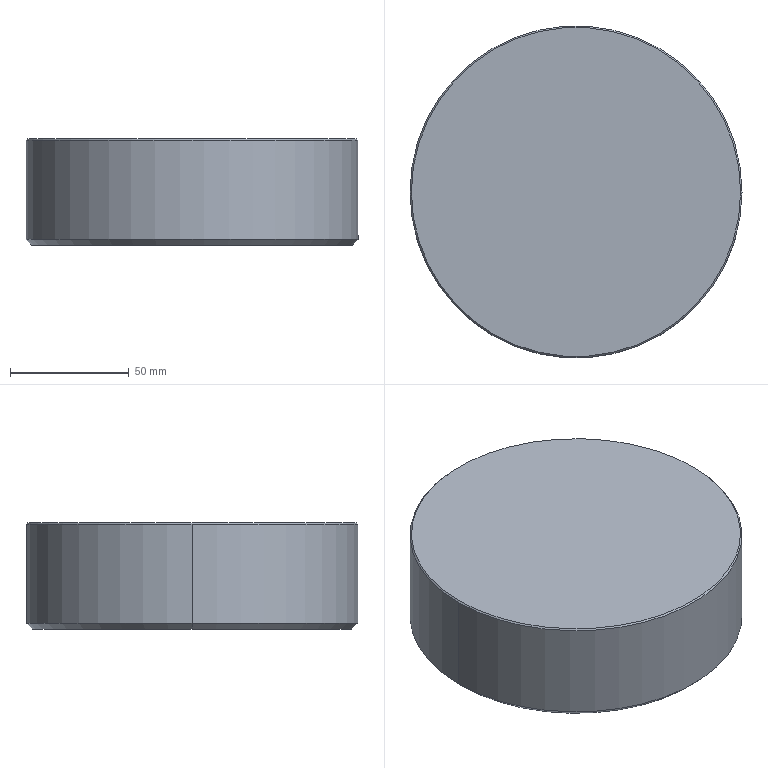Part | SolidWorks | features BaseBody 1 | 1 solid | 13 faces | box 140 x 140 x 45 mm | volume 200339 mm3 | cone 6 | cylinder 4 | plane 3 | commonest cylinder face diameters 125 x2 140 x2
STEP:
#1=CARTESIAN_POINT('',(69.4,0.,45.));
#2=VERTEX_POINT('',#1);
#3=CARTESIAN_POINT('',(-69.4,0.,45.));
#4=VERTEX_POINT('',#3);
#5=CARTESIAN_POINT('',(0.,0.,45.));
#6=DIRECTION('',(0.,0.,1.));
#7=DIRECTION('',(-1.,0.,0.));
#8=AXIS2_PLACEMENT_3D('',#5,#6,#7);
#9=CIRCLE('',#8,69.4);
#10=EDGE_CURVE('',#2,#4,#9,.T.);
#11=ORIENTED_EDGE('',*,*,#10,.F.);
#12=CARTESIAN_POINT('',(70.,0.,44.4));
#13=VERTEX_POINT('',#12);
#14=CARTESIAN_POINT('',(70.,0.,44.4));
#15=DIRECTION('',(0.7071,0.,-0.7071));
#16=VECTOR('',#15,1000.);
#17=LINE('',#14,#16);
#18=EDGE_CURVE('',#2,#13,#17,.T.);
#19=ORIENTED_EDGE('',*,*,#18,.T.);
#20=CARTESIAN_POINT('',(-70.,0.,44.4));
#21=VERTEX_POINT('',#20);
#22=CARTESIAN_POINT('',(0.,0.,44.4));
#23=DIRECTION('',(0.,0.,1.));
#24=DIRECTION('',(-1.,0.,0.));
#25=AXIS2_PLACEMENT_3D('',#22,#23,#24);
#26=CIRCLE('',#25,70.);
#27=EDGE_CURVE('',#13,#21,#26,.T.);
#28=ORIENTED_EDGE('',*,*,#27,.T.);
#29=CARTESIAN_POINT('',(-70.,0.,44.4));
#30=DIRECTION('',(-0.7071,0.,-0.7071));
#31=VECTOR('',#30,1000.);
#32=LINE('',#29,#31);
#33=EDGE_CURVE('',#4,#21,#32,.T.);
#34=ORIENTED_EDGE('',*,*,#33,.F.);
#35=EDGE_LOOP('',(#11,#19,#28,#34));
#36=FACE_OUTER_BOUND('',#35,.T.);
#37=CARTESIAN_POINT('',(0.,0.,44.4));
#38=DIRECTION('',(0.,0.,-1.));
#39=DIRECTION('',(-1.,0.,0.));
#40=AXIS2_PLACEMENT_3D('',#37,#38,#39);
#41=CONICAL_SURFACE('',#40,70.,0.7854);
#42=ADVANCED_FACE('',(#36),#41,.T.);
#43=ORIENTED_EDGE('',*,*,#27,.F.);
#44=CARTESIAN_POINT('',(70.,0.,2.5));
#45=VERTEX_POINT('',#44);
#46=CARTESIAN_POINT('',(70.,0.,40.));
#47=DIRECTION('',(0.,0.,-1.));
#48=VECTOR('',#47,1000.);
#49=LINE('',#46,#48);
#50=EDGE_CURVE('',#13,#45,#49,.T.);
#51=ORIENTED_EDGE('',*,*,#50,.T.);
#52=CARTESIAN_POINT('',(-70.,0.,2.5));
#53=VERTEX_POINT('',#52);
#54=CARTESIAN_POINT('',(0.,0.,2.5));
#55=DIRECTION('',(0.,0.,1.));
#56=DIRECTION('',(-1.,0.,0.));
#57=AXIS2_PLACEMENT_3D('',#54,#55,#56);
#58=CIRCLE('',#57,70.);
#59=EDGE_CURVE('',#45,#53,#58,.T.);
#60=ORIENTED_EDGE('',*,*,#59,.T.);
#61=CARTESIAN_POINT('',(-70.,0.,40.));
#62=DIRECTION('',(0.,0.,-1.));
#63=VECTOR('',#62,1000.);
#64=LINE('',#61,#63);
#65=EDGE_CURVE('',#21,#53,#64,.T.);
#66=ORIENTED_EDGE('',*,*,#65,.F.);
#67=EDGE_LOOP('',(#43,#51,#60,#66));
#68=FACE_OUTER_BOUND('',#67,.T.);
#69=CARTESIAN_POINT('',(0.,0.,40.));
#70=DIRECTION('',(0.,0.,-1.));
#71=DIRECTION('',(-1.,0.,0.));
#72=AXIS2_PLACEMENT_3D('',#69,#70,#71);
#73=CYLINDRICAL_SURFACE('',#72,70.);
#74=ADVANCED_FACE('',(#68),#73,.T.);
#75=CARTESIAN_POINT('',(67.5,0.,0.));
#76=VERTEX_POINT('',#75);
#77=CARTESIAN_POINT('',(-67.5,0.,0.));
#78=VERTEX_POINT('',#77);
#79=CARTESIAN_POINT('',(0.,0.,0.));
#80=DIRECTION('',(0.,0.,1.));
#81=DIRECTION('',(1.,0.,0.));
#82=AXIS2_PLACEMENT_3D('',#79,#80,#81);
#83=CIRCLE('',#82,67.5);
#84=EDGE_CURVE('',#76,#78,#83,.T.);
#85=ORIENTED_EDGE('',*,*,#84,.T.);
#86=CARTESIAN_POINT('',(-70.,0.,2.5));
#87=DIRECTION('',(-0.7071,0.,0.7071));
#88=VECTOR('',#87,1000.);
#89=LINE('',#86,#88);
#90=EDGE_CURVE('',#78,#53,#89,.T.);
#91=ORIENTED_EDGE('',*,*,#90,.T.);
#92=ORIENTED_EDGE('',*,*,#59,.F.);
#93=CARTESIAN_POINT('',(70.,0.,2.5));
#94=DIRECTION('',(0.7071,0.,0.7071));
#95=VECTOR('',#94,1000.);
#96=LINE('',#93,#95);
#97=EDGE_CURVE('',#76,#45,#96,.T.);
#98=ORIENTED_EDGE('',*,*,#97,.F.);
#99=EDGE_LOOP('',(#85,#91,#92,#98));
#100=FACE_OUTER_BOUND('',#99,.T.);
#101=CARTESIAN_POINT('',(0.,0.,2.5));
#102=DIRECTION('',(0.,0.,1.));
#103=DIRECTION('',(1.,0.,0.));
#104=AXIS2_PLACEMENT_3D('',#101,#102,#103);
#105=CONICAL_SURFACE('',#104,70.,0.7854);
#106=ADVANCED_FACE('',(#100),#105,.T.);
#107=CARTESIAN_POINT('',(62.5,0.,0.6));
#108=VERTEX_POINT('',#107);
#109=CARTESIAN_POINT('',(-62.5,0.,0.6));
#110=VERTEX_POINT('',#109);
#111=CARTESIAN_POINT('',(0.,0.,0.6));
#112=DIRECTION('',(0.,0.,-1.));
#113=DIRECTION('',(1.,0.,0.));
#114=AXIS2_PLACEMENT_3D('',#111,#112,#113);
#115=CIRCLE('',#114,62.5);
#116=EDGE_CURVE('',#108,#110,#115,.T.);
#117=ORIENTED_EDGE('',*,*,#116,.F.);
#118=CARTESIAN_POINT('',(63.1,0.,0.));
#119=VERTEX_POINT('',#118);
#120=CARTESIAN_POINT('',(63.1,0.,0.));
#121=DIRECTION('',(0.7071,0.,-0.7071));
#122=VECTOR('',#121,1000.);
#123=LINE('',#120,#122);
#124=EDGE_CURVE('',#108,#119,#123,.T.);
#125=ORIENTED_EDGE('',*,*,#124,.T.);
#126=CARTESIAN_POINT('',(-63.1,0.,0.));
#127=VERTEX_POINT('',#126);
#128=CARTESIAN_POINT('',(0.,0.,0.));
#129=DIRECTION('',(0.,0.,-1.));
#130=DIRECTION('',(-1.,0.,0.));
#131=AXIS2_PLACEMENT_3D('',#128,#129,#130);
#132=CIRCLE('',#131,63.1);
#133=EDGE_CURVE('',#119,#127,#132,.T.);
#134=ORIENTED_EDGE('',*,*,#133,.T.);
#135=CARTESIAN_POINT('',(-63.1,0.,0.));
#136=DIRECTION('',(-0.7071,0.,-0.7071));
#137=VECTOR('',#136,1000.);
#138=LINE('',#135,#137);
#139=EDGE_CURVE('',#110,#127,#138,.T.);
#140=ORIENTED_EDGE('',*,*,#139,.F.);
#141=EDGE_LOOP('',(#117,#125,#134,#140));
#142=FACE_OUTER_BOUND('',#141,.T.);
#143=CARTESIAN_POINT('',(0.,0.,0.));
#144=DIRECTION('',(0.,0.,-1.));
#145=DIRECTION('',(-1.,0.,0.));
#146=AXIS2_PLACEMENT_3D('',#143,#144,#145);
#147=CONICAL_SURFACE('',#146,63.1,0.7854);
#148=ADVANCED_FACE('',(#142),#147,.F.);
#149=CARTESIAN_POINT('',(62.5,0.,40.));
#150=VERTEX_POINT('',#149);
#151=CARTESIAN_POINT('',(-62.5,0.,40.));
#152=VERTEX_POINT('',#151);
#153=CARTESIAN_POINT('',(0.,0.,40.));
#154=DIRECTION('',(0.,0.,-1.));
#155=DIRECTION('',(-1.,0.,0.));
#156=AXIS2_PLACEMENT_3D('',#153,#154,#155);
#157=CIRCLE('',#156,62.5);
#158=EDGE_CURVE('',#150,#152,#157,.T.);
#159=ORIENTED_EDGE('',*,*,#158,.F.);
#160=CARTESIAN_POINT('',(62.5,0.,40.));
#161=DIRECTION('',(0.,0.,-1.));
#162=VECTOR('',#161,1000.);
#163=LINE('',#160,#162);
#164=EDGE_CURVE('',#150,#108,#163,.T.);
#165=ORIENTED_EDGE('',*,*,#164,.T.);
#166=ORIENTED_EDGE('',*,*,#116,.T.);
#167=CARTESIAN_POINT('',(-62.5,0.,40.));
#168=DIRECTION('',(0.,0.,-1.));
#169=VECTOR('',#168,1000.);
#170=LINE('',#167,#169);
#171=EDGE_CURVE('',#152,#110,#170,.T.);
#172=ORIENTED_EDGE('',*,*,#171,.F.);
#173=EDGE_LOOP('',(#159,#165,#166,#172));
#174=FACE_OUTER_BOUND('',#173,.T.);
#175=CARTESIAN_POINT('',(0.,0.,40.));
#176=DIRECTION('',(0.,0.,-1.));
#177=DIRECTION('',(-1.,0.,0.));
#178=AXIS2_PLACEMENT_3D('',#175,#176,#177);
#179=CYLINDRICAL_SURFACE('',#178,62.5);
#180=ADVANCED_FACE('',(#174),#179,.F.);
#181=CARTESIAN_POINT('',(0.,0.,45.));
#182=DIRECTION('',(0.,0.,1.));
#183=DIRECTION('',(-1.,0.,0.));
#184=AXIS2_PLACEMENT_3D('',#181,#182,#183);
#185=CIRCLE('',#184,69.4);
#186=EDGE_CURVE('',#4,#2,#185,.T.);
#187=ORIENTED_EDGE('',*,*,#186,.T.);
#188=ORIENTED_EDGE('',*,*,#10,.T.);
#189=EDGE_LOOP('',(#187,#188));
#190=FACE_OUTER_BOUND('',#189,.T.);
#191=CARTESIAN_POINT('',(0.,0.,45.));
#192=DIRECTION('',(0.,0.,1.));
#193=DIRECTION('',(1.,0.,0.));
#194=AXIS2_PLACEMENT_3D('',#191,#192,#193);
#195=PLANE('',#194);
#196=ADVANCED_FACE('',(#190),#195,.T.);
#197=ORIENTED_EDGE('',*,*,#18,.F.);
#198=ORIENTED_EDGE('',*,*,#186,.F.);
#199=ORIENTED_EDGE('',*,*,#33,.T.);
#200=CARTESIAN_POINT('',(0.,0.,44.4));
#201=DIRECTION('',(0.,0.,1.));
#202=DIRECTION('',(-1.,0.,0.));
#203=AXIS2_PLACEMENT_3D('',#200,#201,#202);
#204=CIRCLE('',#203,70.);
#205=EDGE_CURVE('',#21,#13,#204,.T.);
#206=ORIENTED_EDGE('',*,*,#205,.T.);
#207=EDGE_LOOP('',(#197,#198,#199,#206));
#208=FACE_OUTER_BOUND('',#207,.T.);
#209=CARTESIAN_POINT('',(0.,0.,44.4));
#210=DIRECTION('',(0.,0.,-1.));
#211=DIRECTION('',(-1.,0.,0.));
#212=AXIS2_PLACEMENT_3D('',#209,#210,#211);
#213=CONICAL_SURFACE('',#212,70.,0.7854);
#214=ADVANCED_FACE('',(#208),#213,.T.);
#215=ORIENTED_EDGE('',*,*,#50,.F.);
#216=ORIENTED_EDGE('',*,*,#205,.F.);
#217=ORIENTED_EDGE('',*,*,#65,.T.);
#218=CARTESIAN_POINT('',(0.,0.,2.5));
#219=DIRECTION('',(0.,0.,1.));
#220=DIRECTION('',(-1.,0.,0.));
#221=AXIS2_PLACEMENT_3D('',#218,#219,#220);
#222=CIRCLE('',#221,70.);
#223=EDGE_CURVE('',#53,#45,#222,.T.);
#224=ORIENTED_EDGE('',*,*,#223,.T.);
#225=EDGE_LOOP('',(#215,#216,#217,#224));
#226=FACE_OUTER_BOUND('',#225,.T.);
#227=CARTESIAN_POINT('',(0.,0.,40.));
#228=DIRECTION('',(0.,0.,-1.));
#229=DIRECTION('',(-1.,0.,0.));
#230=AXIS2_PLACEMENT_3D('',#227,#228,#229);
#231=CYLINDRICAL_SURFACE('',#230,70.);
#232=ADVANCED_FACE('',(#226),#231,.T.);
#233=ORIENTED_EDGE('',*,*,#90,.F.);
#234=CARTESIAN_POINT('',(0.,0.,0.));
#235=DIRECTION('',(0.,0.,1.));
#236=DIRECTION('',(1.,0.,0.));
#237=AXIS2_PLACEMENT_3D('',#234,#235,#236);
#238=CIRCLE('',#237,67.5);
#239=EDGE_CURVE('',#78,#76,#238,.T.);
#240=ORIENTED_EDGE('',*,*,#239,.T.);
#241=ORIENTED_EDGE('',*,*,#97,.T.);
#242=ORIENTED_EDGE('',*,*,#223,.F.);
#243=EDGE_LOOP('',(#233,#240,#241,#242));
#244=FACE_OUTER_BOUND('',#243,.T.);
#245=CARTESIAN_POINT('',(0.,0.,2.5));
#246=DIRECTION('',(0.,0.,1.));
#247=DIRECTION('',(1.,0.,0.));
#248=AXIS2_PLACEMENT_3D('',#245,#246,#247);
#249=CONICAL_SURFACE('',#248,70.,0.7854);
#250=ADVANCED_FACE('',(#244),#249,.T.);
#251=CARTESIAN_POINT('',(0.,0.,0.));
#252=DIRECTION('',(0.,0.,-1.));
#253=DIRECTION('',(-1.,0.,0.));
#254=AXIS2_PLACEMENT_3D('',#251,#252,#253);
#255=CIRCLE('',#254,63.1);
#256=EDGE_CURVE('',#127,#119,#255,.T.);
#257=ORIENTED_EDGE('',*,*,#256,.F.);
#258=ORIENTED_EDGE('',*,*,#133,.F.);
#259=EDGE_LOOP('',(#257,#258));
#260=FACE_BOUND('',#259,.T.);
#261=ORIENTED_EDGE('',*,*,#84,.F.);
#262=ORIENTED_EDGE('',*,*,#239,.F.);
#263=EDGE_LOOP('',(#261,#262));
#264=FACE_OUTER_BOUND('',#263,.T.);
#265=CARTESIAN_POINT('',(0.,0.,0.));
#266=DIRECTION('',(0.,0.,1.));
#267=DIRECTION('',(1.,0.,0.));
#268=AXIS2_PLACEMENT_3D('',#265,#266,#267);
#269=PLANE('',#268);
#270=ADVANCED_FACE('',(#260,#264),#269,.F.);
#271=ORIENTED_EDGE('',*,*,#124,.F.);
#272=CARTESIAN_POINT('',(0.,0.,0.6));
#273=DIRECTION('',(0.,0.,-1.));
#274=DIRECTION('',(1.,0.,0.));
#275=AXIS2_PLACEMENT_3D('',#272,#273,#274);
#276=CIRCLE('',#275,62.5);
#277=EDGE_CURVE('',#110,#108,#276,.T.);
#278=ORIENTED_EDGE('',*,*,#277,.F.);
#279=ORIENTED_EDGE('',*,*,#139,.T.);
#280=ORIENTED_EDGE('',*,*,#256,.T.);
#281=EDGE_LOOP('',(#271,#278,#279,#280));
#282=FACE_OUTER_BOUND('',#281,.T.);
#283=CARTESIAN_POINT('',(0.,0.,0.));
#284=DIRECTION('',(0.,0.,-1.));
#285=DIRECTION('',(-1.,0.,0.));
#286=AXIS2_PLACEMENT_3D('',#283,#284,#285);
#287=CONICAL_SURFACE('',#286,63.1,0.7854);
#288=ADVANCED_FACE('',(#282),#287,.F.);
#289=ORIENTED_EDGE('',*,*,#164,.F.);
#290=CARTESIAN_POINT('',(0.,0.,40.));
#291=DIRECTION('',(0.,0.,-1.));
#292=DIRECTION('',(-1.,0.,0.));
#293=AXIS2_PLACEMENT_3D('',#290,#291,#292);
#294=CIRCLE('',#293,62.5);
#295=EDGE_CURVE('',#152,#150,#294,.T.);
#296=ORIENTED_EDGE('',*,*,#295,.F.);
#297=ORIENTED_EDGE('',*,*,#171,.T.);
#298=ORIENTED_EDGE('',*,*,#277,.T.);
#299=EDGE_LOOP('',(#289,#296,#297,#298));
#300=FACE_OUTER_BOUND('',#299,.T.);
#301=CARTESIAN_POINT('',(0.,0.,40.));
#302=DIRECTION('',(0.,0.,-1.));
#303=DIRECTION('',(-1.,0.,0.));
#304=AXIS2_PLACEMENT_3D('',#301,#302,#303);
#305=CYLINDRICAL_SURFACE('',#304,62.5);
#306=ADVANCED_FACE('',(#300),#305,.F.);
#307=ORIENTED_EDGE('',*,*,#295,.T.);
#308=ORIENTED_EDGE('',*,*,#158,.T.);
#309=EDGE_LOOP('',(#307,#308));
#310=FACE_OUTER_BOUND('',#309,.T.);
#311=CARTESIAN_POINT('',(0.,0.,40.));
#312=DIRECTION('',(0.,0.,1.));
#313=DIRECTION('',(1.,0.,0.));
#314=AXIS2_PLACEMENT_3D('',#311,#312,#313);
#315=PLANE('',#314);
#316=ADVANCED_FACE('',(#310),#315,.F.);
#317=CLOSED_SHELL('',(#42,#74,#106,#148,#180,#196,#214,#232,#250,#270,#288,#306,#316));
#318=MANIFOLD_SOLID_BREP('',#317);
#319=CARTESIAN_POINT('',(0.,0.,0.));
#320=DIRECTION('',(0.,0.,1.));
#321=DIRECTION('',(1.,0.,0.));
#322=AXIS2_PLACEMENT_3D('',#319,#320,#321);
#323=(LENGTH_UNIT()NAMED_UNIT(*)SI_UNIT(.MILLI.,.METRE.));
#324=UNCERTAINTY_MEASURE_WITH_UNIT(LENGTH_MEASURE(0.00001),#323,'','');
#325=(NAMED_UNIT(*)PLANE_ANGLE_UNIT()SI_UNIT($,.RADIAN.));
#326=(NAMED_UNIT(*)SI_UNIT($,.STERADIAN.)SOLID_ANGLE_UNIT());
#327=(GEOMETRIC_REPRESENTATION_CONTEXT(3)GLOBAL_UNCERTAINTY_ASSIGNED_CONTEXT((#324))GLOBAL_UNIT_ASSIGNED_CONTEXT((#323,#325,#326))REPRESENTATION_CONTEXT('',''));
#328=ADVANCED_BREP_SHAPE_REPRESENTATION('',(#318,#322),#327);